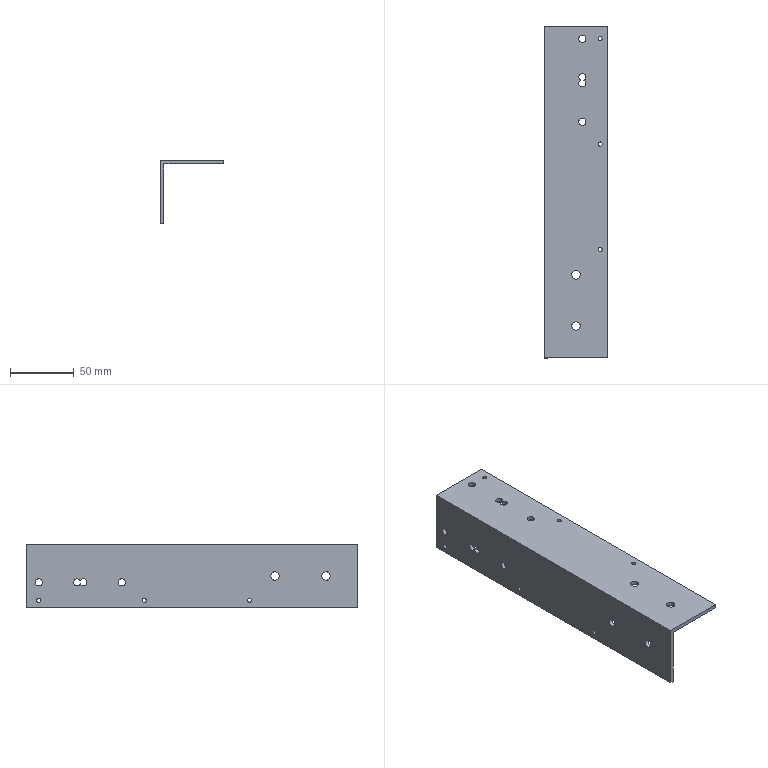Part | SolidWorks | features HoleWzd 6, CirPattern 1, Extrusion 1 | 1 solid | 48 faces | box 50 x 260 x 50 mm | volume 74530 mm3 | cylinder 40 | plane 8 | commonest cylinder face diameters 5.5 x20 3.3 x12 6.6 x8